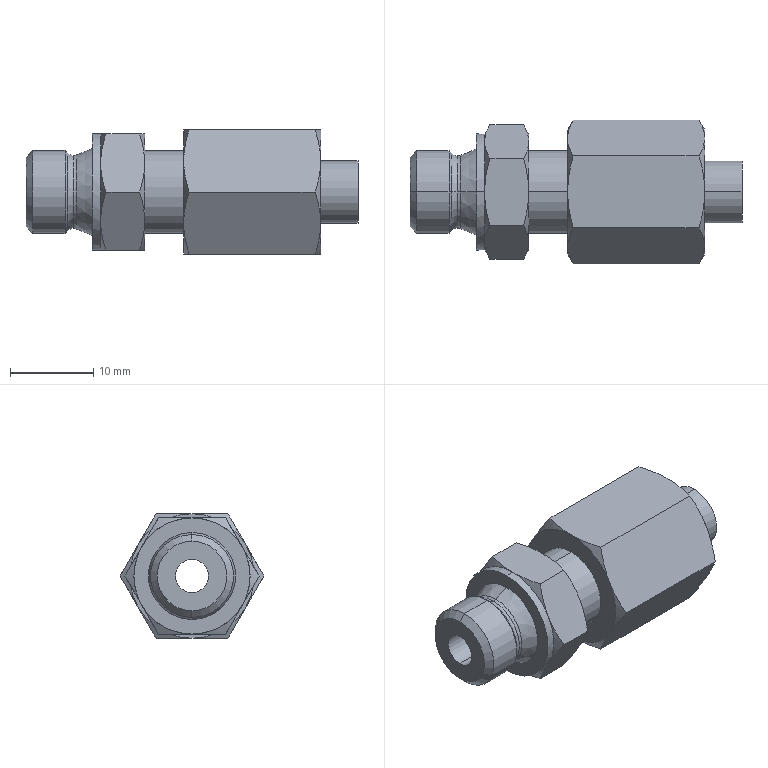Part | SolidWorks | features ICE 2, Boss 1, RevCut 1, Revolution 1 | 1 solid | 65 faces | box 40 x 17.321 x 15 mm | volume 4755 mm3 | cone 30 | plane 19 | cylinder 12 | torus 4 | commonest cylinder face diameters 10 x4 4 x2 6 x2 7.5 x2 14 x2